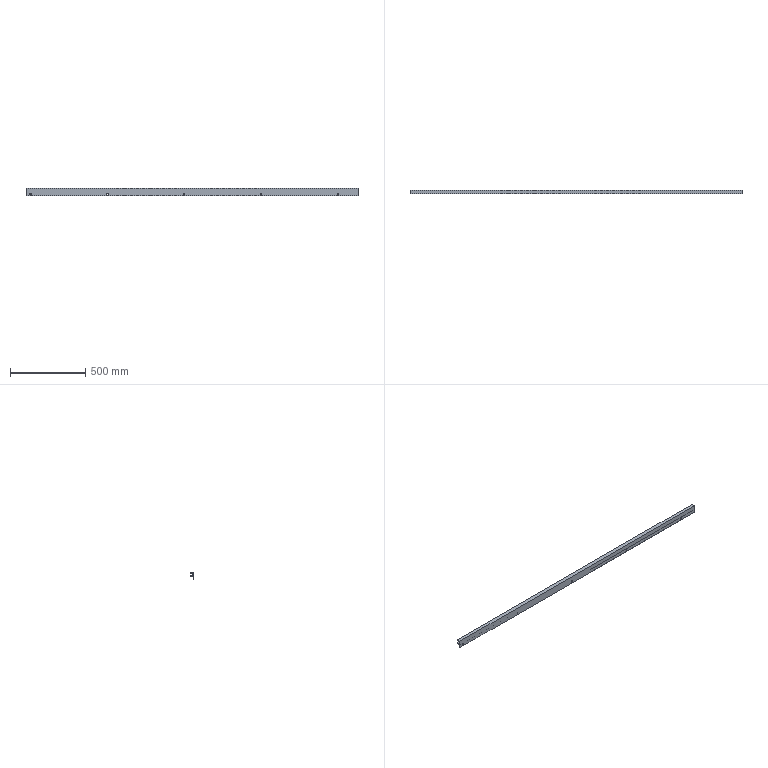Part | SolidWorks | features ICE 3, Extrusion 1, LPattern 1 | 1 solid | 45 faces | box 2200 x 24 x 52 mm | volume 1222839 mm3 | plane 30 | cylinder 15 | commonest cylinder face diameters 7 x15
STEP:
#1=CARTESIAN_POINT('',(540.,-9.,-33.5));
#2=VERTEX_POINT('',#1);
#3=CARTESIAN_POINT('',(543.5,-9.,-30.));
#4=VERTEX_POINT('',#3);
#5=CARTESIAN_POINT('',(540.,-9.,-30.));
#6=DIRECTION('',(0.,-1.,0.));
#7=DIRECTION('',(0.,0.,-1.));
#8=AXIS2_PLACEMENT_3D('',#5,#6,#7);
#9=CIRCLE('',#8,3.5);
#10=EDGE_CURVE('',#2,#4,#9,.T.);
#11=ORIENTED_EDGE('',*,*,#10,.F.);
#12=CARTESIAN_POINT('',(540.,-12.,-33.5));
#13=VERTEX_POINT('',#12);
#14=CARTESIAN_POINT('',(540.,10.,-33.5));
#15=DIRECTION('',(0.,-1.,0.));
#16=VECTOR('',#15,1000.);
#17=LINE('',#14,#16);
#18=EDGE_CURVE('',#2,#13,#17,.T.);
#19=ORIENTED_EDGE('',*,*,#18,.T.);
#20=CARTESIAN_POINT('',(543.5,-12.,-30.));
#21=VERTEX_POINT('',#20);
#22=CARTESIAN_POINT('',(540.,-12.,-30.));
#23=DIRECTION('',(0.,-1.,0.));
#24=DIRECTION('',(0.,0.,-1.));
#25=AXIS2_PLACEMENT_3D('',#22,#23,#24);
#26=CIRCLE('',#25,3.5);
#27=EDGE_CURVE('',#13,#21,#26,.T.);
#28=ORIENTED_EDGE('',*,*,#27,.T.);
#29=CARTESIAN_POINT('',(543.5,10.,-30.));
#30=DIRECTION('',(0.,-1.,0.));
#31=VECTOR('',#30,1000.);
#32=LINE('',#29,#31);
#33=EDGE_CURVE('',#4,#21,#32,.T.);
#34=ORIENTED_EDGE('',*,*,#33,.F.);
#35=EDGE_LOOP('',(#11,#19,#28,#34));
#36=FACE_OUTER_BOUND('',#35,.T.);
#37=CARTESIAN_POINT('',(540.,10.,-30.));
#38=DIRECTION('',(0.,-1.,0.));
#39=DIRECTION('',(0.,0.,-1.));
#40=AXIS2_PLACEMENT_3D('',#37,#38,#39);
#41=CYLINDRICAL_SURFACE('',#40,3.5);
#42=ADVANCED_FACE('',(#36),#41,.F.);
#43=CARTESIAN_POINT('',(1050.,-9.,-33.5));
#44=VERTEX_POINT('',#43);
#45=CARTESIAN_POINT('',(1053.5,-9.,-30.));
#46=VERTEX_POINT('',#45);
#47=CARTESIAN_POINT('',(1050.,-9.,-30.));
#48=DIRECTION('',(0.,-1.,0.));
#49=DIRECTION('',(0.,0.,-1.));
#50=AXIS2_PLACEMENT_3D('',#47,#48,#49);
#51=CIRCLE('',#50,3.5);
#52=EDGE_CURVE('',#44,#46,#51,.T.);
#53=ORIENTED_EDGE('',*,*,#52,.F.);
#54=CARTESIAN_POINT('',(1050.,-12.,-33.5));
#55=VERTEX_POINT('',#54);
#56=CARTESIAN_POINT('',(1050.,10.,-33.5));
#57=DIRECTION('',(0.,-1.,0.));
#58=VECTOR('',#57,1000.);
#59=LINE('',#56,#58);
#60=EDGE_CURVE('',#44,#55,#59,.T.);
#61=ORIENTED_EDGE('',*,*,#60,.T.);
#62=CARTESIAN_POINT('',(1053.5,-12.,-30.));
#63=VERTEX_POINT('',#62);
#64=CARTESIAN_POINT('',(1050.,-12.,-30.));
#65=DIRECTION('',(0.,-1.,0.));
#66=DIRECTION('',(0.,0.,-1.));
#67=AXIS2_PLACEMENT_3D('',#64,#65,#66);
#68=CIRCLE('',#67,3.5);
#69=EDGE_CURVE('',#55,#63,#68,.T.);
#70=ORIENTED_EDGE('',*,*,#69,.T.);
#71=CARTESIAN_POINT('',(1053.5,10.,-30.));
#72=DIRECTION('',(0.,-1.,0.));
#73=VECTOR('',#72,1000.);
#74=LINE('',#71,#73);
#75=EDGE_CURVE('',#46,#63,#74,.T.);
#76=ORIENTED_EDGE('',*,*,#75,.F.);
#77=EDGE_LOOP('',(#53,#61,#70,#76));
#78=FACE_OUTER_BOUND('',#77,.T.);
#79=CARTESIAN_POINT('',(1050.,10.,-30.));
#80=DIRECTION('',(0.,-1.,0.));
#81=DIRECTION('',(0.,0.,-1.));
#82=AXIS2_PLACEMENT_3D('',#79,#80,#81);
#83=CYLINDRICAL_SURFACE('',#82,3.5);
#84=ADVANCED_FACE('',(#78),#83,.F.);
#85=CARTESIAN_POINT('',(1560.,-9.,-33.5));
#86=VERTEX_POINT('',#85);
#87=CARTESIAN_POINT('',(1563.5,-9.,-30.));
#88=VERTEX_POINT('',#87);
#89=CARTESIAN_POINT('',(1560.,-9.,-30.));
#90=DIRECTION('',(0.,-1.,0.));
#91=DIRECTION('',(0.,0.,-1.));
#92=AXIS2_PLACEMENT_3D('',#89,#90,#91);
#93=CIRCLE('',#92,3.5);
#94=EDGE_CURVE('',#86,#88,#93,.T.);
#95=ORIENTED_EDGE('',*,*,#94,.F.);
#96=CARTESIAN_POINT('',(1560.,-12.,-33.5));
#97=VERTEX_POINT('',#96);
#98=CARTESIAN_POINT('',(1560.,10.,-33.5));
#99=DIRECTION('',(0.,-1.,0.));
#100=VECTOR('',#99,1000.);
#101=LINE('',#98,#100);
#102=EDGE_CURVE('',#86,#97,#101,.T.);
#103=ORIENTED_EDGE('',*,*,#102,.T.);
#104=CARTESIAN_POINT('',(1563.5,-12.,-30.));
#105=VERTEX_POINT('',#104);
#106=CARTESIAN_POINT('',(1560.,-12.,-30.));
#107=DIRECTION('',(0.,-1.,0.));
#108=DIRECTION('',(0.,0.,-1.));
#109=AXIS2_PLACEMENT_3D('',#106,#107,#108);
#110=CIRCLE('',#109,3.5);
#111=EDGE_CURVE('',#97,#105,#110,.T.);
#112=ORIENTED_EDGE('',*,*,#111,.T.);
#113=CARTESIAN_POINT('',(1563.5,10.,-30.));
#114=DIRECTION('',(0.,-1.,0.));
#115=VECTOR('',#114,1000.);
#116=LINE('',#113,#115);
#117=EDGE_CURVE('',#88,#105,#116,.T.);
#118=ORIENTED_EDGE('',*,*,#117,.F.);
#119=EDGE_LOOP('',(#95,#103,#112,#118));
#120=FACE_OUTER_BOUND('',#119,.T.);
#121=CARTESIAN_POINT('',(1560.,10.,-30.));
#122=DIRECTION('',(0.,-1.,0.));
#123=DIRECTION('',(0.,0.,-1.));
#124=AXIS2_PLACEMENT_3D('',#121,#122,#123);
#125=CYLINDRICAL_SURFACE('',#124,3.5);
#126=ADVANCED_FACE('',(#120),#125,.F.);
#127=CARTESIAN_POINT('',(2070.,-9.,-33.5));
#128=VERTEX_POINT('',#127);
#129=CARTESIAN_POINT('',(2073.5,-9.,-30.));
#130=VERTEX_POINT('',#129);
#131=CARTESIAN_POINT('',(2070.,-9.,-30.));
#132=DIRECTION('',(0.,-1.,0.));
#133=DIRECTION('',(0.,0.,-1.));
#134=AXIS2_PLACEMENT_3D('',#131,#132,#133);
#135=CIRCLE('',#134,3.5);
#136=EDGE_CURVE('',#128,#130,#135,.T.);
#137=ORIENTED_EDGE('',*,*,#136,.F.);
#138=CARTESIAN_POINT('',(2070.,-12.,-33.5));
#139=VERTEX_POINT('',#138);
#140=CARTESIAN_POINT('',(2070.,10.,-33.5));
#141=DIRECTION('',(0.,-1.,0.));
#142=VECTOR('',#141,1000.);
#143=LINE('',#140,#142);
#144=EDGE_CURVE('',#128,#139,#143,.T.);
#145=ORIENTED_EDGE('',*,*,#144,.T.);
#146=CARTESIAN_POINT('',(2073.5,-12.,-30.));
#147=VERTEX_POINT('',#146);
#148=CARTESIAN_POINT('',(2070.,-12.,-30.));
#149=DIRECTION('',(0.,-1.,0.));
#150=DIRECTION('',(0.,0.,-1.));
#151=AXIS2_PLACEMENT_3D('',#148,#149,#150);
#152=CIRCLE('',#151,3.5);
#153=EDGE_CURVE('',#139,#147,#152,.T.);
#154=ORIENTED_EDGE('',*,*,#153,.T.);
#155=CARTESIAN_POINT('',(2073.5,10.,-30.));
#156=DIRECTION('',(0.,-1.,0.));
#157=VECTOR('',#156,1000.);
#158=LINE('',#155,#157);
#159=EDGE_CURVE('',#130,#147,#158,.T.);
#160=ORIENTED_EDGE('',*,*,#159,.F.);
#161=EDGE_LOOP('',(#137,#145,#154,#160));
#162=FACE_OUTER_BOUND('',#161,.T.);
#163=CARTESIAN_POINT('',(2070.,10.,-30.));
#164=DIRECTION('',(0.,-1.,0.));
#165=DIRECTION('',(0.,0.,-1.));
#166=AXIS2_PLACEMENT_3D('',#163,#164,#165);
#167=CYLINDRICAL_SURFACE('',#166,3.5);
#168=ADVANCED_FACE('',(#162),#167,.F.);
#169=CARTESIAN_POINT('',(30.,-9.,-33.5));
#170=VERTEX_POINT('',#169);
#171=CARTESIAN_POINT('',(33.5,-9.,-30.));
#172=VERTEX_POINT('',#171);
#173=CARTESIAN_POINT('',(30.,-9.,-30.));
#174=DIRECTION('',(0.,-1.,0.));
#175=DIRECTION('',(0.,0.,-1.));
#176=AXIS2_PLACEMENT_3D('',#173,#174,#175);
#177=CIRCLE('',#176,3.5);
#178=EDGE_CURVE('',#170,#172,#177,.T.);
#179=ORIENTED_EDGE('',*,*,#178,.F.);
#180=CARTESIAN_POINT('',(30.,-12.,-33.5));
#181=VERTEX_POINT('',#180);
#182=CARTESIAN_POINT('',(30.,10.,-33.5));
#183=DIRECTION('',(0.,-1.,0.));
#184=VECTOR('',#183,1000.);
#185=LINE('',#182,#184);
#186=EDGE_CURVE('',#170,#181,#185,.T.);
#187=ORIENTED_EDGE('',*,*,#186,.T.);
#188=CARTESIAN_POINT('',(33.5,-12.,-30.));
#189=VERTEX_POINT('',#188);
#190=CARTESIAN_POINT('',(30.,-12.,-30.));
#191=DIRECTION('',(0.,-1.,0.));
#192=DIRECTION('',(0.,0.,-1.));
#193=AXIS2_PLACEMENT_3D('',#190,#191,#192);
#194=CIRCLE('',#193,3.5);
#195=EDGE_CURVE('',#181,#189,#194,.T.);
#196=ORIENTED_EDGE('',*,*,#195,.T.);
#197=CARTESIAN_POINT('',(33.5,10.,-30.));
#198=DIRECTION('',(0.,-1.,0.));
#199=VECTOR('',#198,1000.);
#200=LINE('',#197,#199);
#201=EDGE_CURVE('',#172,#189,#200,.T.);
#202=ORIENTED_EDGE('',*,*,#201,.F.);
#203=EDGE_LOOP('',(#179,#187,#196,#202));
#204=FACE_OUTER_BOUND('',#203,.T.);
#205=CARTESIAN_POINT('',(30.,10.,-30.));
#206=DIRECTION('',(0.,-1.,0.));
#207=DIRECTION('',(0.,0.,-1.));
#208=AXIS2_PLACEMENT_3D('',#205,#206,#207);
#209=CYLINDRICAL_SURFACE('',#208,3.5);
#210=ADVANCED_FACE('',(#204),#209,.F.);
#211=CARTESIAN_POINT('',(0.,-9.,-15.));
#212=VERTEX_POINT('',#211);
#213=CARTESIAN_POINT('',(2200.,-9.,-15.));
#214=VERTEX_POINT('',#213);
#215=CARTESIAN_POINT('',(2200.,-9.,-15.));
#216=DIRECTION('',(1.,0.,0.));
#217=VECTOR('',#216,1000.);
#218=LINE('',#215,#217);
#219=EDGE_CURVE('',#212,#214,#218,.T.);
#220=ORIENTED_EDGE('',*,*,#219,.F.);
#221=CARTESIAN_POINT('',(0.,12.,-15.));
#222=VERTEX_POINT('',#221);
#223=CARTESIAN_POINT('',(0.,12.,-15.));
#224=DIRECTION('',(0.,1.,0.));
#225=VECTOR('',#224,1000.);
#226=LINE('',#223,#225);
#227=EDGE_CURVE('',#212,#222,#226,.T.);
#228=ORIENTED_EDGE('',*,*,#227,.T.);
#229=CARTESIAN_POINT('',(2200.,12.,-15.));
#230=VERTEX_POINT('',#229);
#231=CARTESIAN_POINT('',(2200.,12.,-15.));
#232=DIRECTION('',(-1.,0.,0.));
#233=VECTOR('',#232,1000.);
#234=LINE('',#231,#233);
#235=EDGE_CURVE('',#230,#222,#234,.T.);
#236=ORIENTED_EDGE('',*,*,#235,.F.);
#237=CARTESIAN_POINT('',(2200.,12.,-15.));
#238=DIRECTION('',(0.,1.,0.));
#239=VECTOR('',#238,1000.);
#240=LINE('',#237,#239);
#241=EDGE_CURVE('',#214,#230,#240,.T.);
#242=ORIENTED_EDGE('',*,*,#241,.F.);
#243=EDGE_LOOP('',(#220,#228,#236,#242));
#244=FACE_OUTER_BOUND('',#243,.T.);
#245=CARTESIAN_POINT('',(2200.,12.,-15.));
#246=DIRECTION('',(0.,0.,1.));
#247=DIRECTION('',(0.,-1.,0.));
#248=AXIS2_PLACEMENT_3D('',#245,#246,#247);
#249=PLANE('',#248);
#250=ADVANCED_FACE('',(#244),#249,.F.);
#251=CARTESIAN_POINT('',(0.,12.,-6.2));
#252=VERTEX_POINT('',#251);
#253=CARTESIAN_POINT('',(2200.,12.,-6.2));
#254=VERTEX_POINT('',#253);
#255=CARTESIAN_POINT('',(0.,12.,-6.2));
#256=DIRECTION('',(1.,0.,0.));
#257=VECTOR('',#256,1000.);
#258=LINE('',#255,#257);
#259=EDGE_CURVE('',#252,#254,#258,.T.);
#260=ORIENTED_EDGE('',*,*,#259,.T.);
#261=CARTESIAN_POINT('',(2200.,12.,15.));
#262=DIRECTION('',(0.,0.,1.));
#263=VECTOR('',#262,1000.);
#264=LINE('',#261,#263);
#265=EDGE_CURVE('',#230,#254,#264,.T.);
#266=ORIENTED_EDGE('',*,*,#265,.F.);
#267=ORIENTED_EDGE('',*,*,#235,.T.);
#268=CARTESIAN_POINT('',(0.,12.,15.));
#269=DIRECTION('',(0.,0.,1.));
#270=VECTOR('',#269,1000.);
#271=LINE('',#268,#270);
#272=EDGE_CURVE('',#222,#252,#271,.T.);
#273=ORIENTED_EDGE('',*,*,#272,.T.);
#274=EDGE_LOOP('',(#260,#266,#267,#273));
#275=FACE_OUTER_BOUND('',#274,.T.);
#276=CARTESIAN_POINT('',(2200.,12.,15.));
#277=DIRECTION('',(0.,-1.,0.));
#278=DIRECTION('',(0.,0.,-1.));
#279=AXIS2_PLACEMENT_3D('',#276,#277,#278);
#280=PLANE('',#279);
#281=ADVANCED_FACE('',(#275),#280,.F.);
#282=ORIENTED_EDGE('',*,*,#265,.T.);
#283=CARTESIAN_POINT('',(2200.,0.7,-6.2));
#284=VERTEX_POINT('',#283);
#285=CARTESIAN_POINT('',(2200.,12.,-6.2));
#286=DIRECTION('',(0.,-1.,0.));
#287=VECTOR('',#286,1000.);
#288=LINE('',#285,#287);
#289=EDGE_CURVE('',#254,#284,#288,.T.);
#290=ORIENTED_EDGE('',*,*,#289,.T.);
#291=CARTESIAN_POINT('',(2200.,0.7,-8.5));
#292=VERTEX_POINT('',#291);
#293=CARTESIAN_POINT('',(2200.,0.7,-6.2));
#294=DIRECTION('',(0.,0.,-1.));
#295=VECTOR('',#294,1000.);
#296=LINE('',#293,#295);
#297=EDGE_CURVE('',#284,#292,#296,.T.);
#298=ORIENTED_EDGE('',*,*,#297,.T.);
#299=CARTESIAN_POINT('',(2200.,-3.9,-8.5));
#300=VERTEX_POINT('',#299);
#301=CARTESIAN_POINT('',(2200.,0.7,-8.5));
#302=DIRECTION('',(0.,-1.,0.));
#303=VECTOR('',#302,1000.);
#304=LINE('',#301,#303);
#305=EDGE_CURVE('',#292,#300,#304,.T.);
#306=ORIENTED_EDGE('',*,*,#305,.T.);
#307=CARTESIAN_POINT('',(2200.,-3.9,-3.5));
#308=VERTEX_POINT('',#307);
#309=CARTESIAN_POINT('',(2200.,-3.9,-8.5));
#310=DIRECTION('',(0.,0.,1.));
#311=VECTOR('',#310,1000.);
#312=LINE('',#309,#311);
#313=EDGE_CURVE('',#300,#308,#312,.T.);
#314=ORIENTED_EDGE('',*,*,#313,.T.);
#315=CARTESIAN_POINT('',(2200.,-5.5,-3.5));
#316=VERTEX_POINT('',#315);
#317=CARTESIAN_POINT('',(2200.,-3.9,-3.5));
#318=DIRECTION('',(0.,-1.,0.));
#319=VECTOR('',#318,1000.);
#320=LINE('',#317,#319);
#321=EDGE_CURVE('',#308,#316,#320,.T.);
#322=ORIENTED_EDGE('',*,*,#321,.T.);
#323=CARTESIAN_POINT('',(2200.,-5.5,3.5));
#324=VERTEX_POINT('',#323);
#325=CARTESIAN_POINT('',(2200.,-5.5,3.5));
#326=DIRECTION('',(0.,0.,-1.));
#327=VECTOR('',#326,1000.);
#328=LINE('',#325,#327);
#329=EDGE_CURVE('',#324,#316,#328,.T.);
#330=ORIENTED_EDGE('',*,*,#329,.F.);
#331=CARTESIAN_POINT('',(2200.,-3.9,3.5));
#332=VERTEX_POINT('',#331);
#333=CARTESIAN_POINT('',(2200.,-3.9,3.5));
#334=DIRECTION('',(0.,-1.,0.));
#335=VECTOR('',#334,1000.);
#336=LINE('',#333,#335);
#337=EDGE_CURVE('',#332,#324,#336,.T.);
#338=ORIENTED_EDGE('',*,*,#337,.F.);
#339=CARTESIAN_POINT('',(2200.,-3.9,8.5));
#340=VERTEX_POINT('',#339);
#341=CARTESIAN_POINT('',(2200.,-3.9,8.5));
#342=DIRECTION('',(0.,0.,-1.));
#343=VECTOR('',#342,1000.);
#344=LINE('',#341,#343);
#345=EDGE_CURVE('',#340,#332,#344,.T.);
#346=ORIENTED_EDGE('',*,*,#345,.F.);
#347=CARTESIAN_POINT('',(2200.,0.7,8.5));
#348=VERTEX_POINT('',#347);
#349=CARTESIAN_POINT('',(2200.,0.7,8.5));
#350=DIRECTION('',(0.,-1.,0.));
#351=VECTOR('',#350,1000.);
#352=LINE('',#349,#351);
#353=EDGE_CURVE('',#348,#340,#352,.T.);
#354=ORIENTED_EDGE('',*,*,#353,.F.);
#355=CARTESIAN_POINT('',(2200.,0.7,6.2));
#356=VERTEX_POINT('',#355);
#357=CARTESIAN_POINT('',(2200.,0.7,6.2));
#358=DIRECTION('',(0.,0.,1.));
#359=VECTOR('',#358,1000.);
#360=LINE('',#357,#359);
#361=EDGE_CURVE('',#356,#348,#360,.T.);
#362=ORIENTED_EDGE('',*,*,#361,.F.);
#363=CARTESIAN_POINT('',(2200.,12.,6.2));
#364=VERTEX_POINT('',#363);
#365=CARTESIAN_POINT('',(2200.,12.,6.2));
#366=DIRECTION('',(0.,-1.,0.));
#367=VECTOR('',#366,1000.);
#368=LINE('',#365,#367);
#369=EDGE_CURVE('',#364,#356,#368,.T.);
#370=ORIENTED_EDGE('',*,*,#369,.F.);
#371=CARTESIAN_POINT('',(2200.,12.,15.));
#372=VERTEX_POINT('',#371);
#373=CARTESIAN_POINT('',(2200.,12.,15.));
#374=DIRECTION('',(0.,0.,1.));
#375=VECTOR('',#374,1000.);
#376=LINE('',#373,#375);
#377=EDGE_CURVE('',#364,#372,#376,.T.);
#378=ORIENTED_EDGE('',*,*,#377,.T.);
#379=CARTESIAN_POINT('',(2200.,-12.,15.));
#380=VERTEX_POINT('',#379);
#381=CARTESIAN_POINT('',(2200.,12.,15.));
#382=DIRECTION('',(0.,-1.,0.));
#383=VECTOR('',#382,1000.);
#384=LINE('',#381,#383);
#385=EDGE_CURVE('',#372,#380,#384,.T.);
#386=ORIENTED_EDGE('',*,*,#385,.T.);
#387=CARTESIAN_POINT('',(2200.,-12.,-37.));
#388=VERTEX_POINT('',#387);
#389=CARTESIAN_POINT('',(2200.,-12.,15.));
#390=DIRECTION('',(0.,0.,-1.));
#391=VECTOR('',#390,1000.);
#392=LINE('',#389,#391);
#393=EDGE_CURVE('',#380,#388,#392,.T.);
#394=ORIENTED_EDGE('',*,*,#393,.T.);
#395=CARTESIAN_POINT('',(2200.,-9.,-37.));
#396=VERTEX_POINT('',#395);
#397=CARTESIAN_POINT('',(2200.,-12.,-37.));
#398=DIRECTION('',(0.,-1.,0.));
#399=VECTOR('',#398,1000.);
#400=LINE('',#397,#399);
#401=EDGE_CURVE('',#396,#388,#400,.T.);
#402=ORIENTED_EDGE('',*,*,#401,.F.);
#403=CARTESIAN_POINT('',(2200.,-9.,-37.));
#404=DIRECTION('',(0.,0.,1.));
#405=VECTOR('',#404,1000.);
#406=LINE('',#403,#405);
#407=EDGE_CURVE('',#396,#214,#406,.T.);
#408=ORIENTED_EDGE('',*,*,#407,.T.);
#409=ORIENTED_EDGE('',*,*,#241,.T.);
#410=EDGE_LOOP('',(#282,#290,#298,#306,#314,#322,#330,#338,#346,#354,#362,#370,#378,#386,#394,#402,#408,#409));
#411=FACE_OUTER_BOUND('',#410,.T.);
#412=CARTESIAN_POINT('',(2200.,0.,0.));
#413=DIRECTION('',(1.,0.,0.));
#414=DIRECTION('',(0.,0.,-1.));
#415=AXIS2_PLACEMENT_3D('',#412,#413,#414);
#416=PLANE('',#415);
#417=ADVANCED_FACE('',(#411),#416,.T.);
#418=CARTESIAN_POINT('',(0.,0.7,-6.2));
#419=VERTEX_POINT('',#418);
#420=CARTESIAN_POINT('',(0.,12.,-6.2));
#421=DIRECTION('',(0.,-1.,0.));
#422=VECTOR('',#421,1000.);
#423=LINE('',#420,#422);
#424=EDGE_CURVE('',#252,#419,#423,.T.);
#425=ORIENTED_EDGE('',*,*,#424,.F.);
#426=ORIENTED_EDGE('',*,*,#272,.F.);
#427=ORIENTED_EDGE('',*,*,#227,.F.);
#428=CARTESIAN_POINT('',(0.,-9.,-37.));
#429=VERTEX_POINT('',#428);
#430=CARTESIAN_POINT('',(0.,-9.,-37.));
#431=DIRECTION('',(0.,0.,1.));
#432=VECTOR('',#431,1000.);
#433=LINE('',#430,#432);
#434=EDGE_CURVE('',#429,#212,#433,.T.);
#435=ORIENTED_EDGE('',*,*,#434,.F.);
#436=CARTESIAN_POINT('',(0.,-12.,-37.));
#437=VERTEX_POINT('',#436);
#438=CARTESIAN_POINT('',(0.,-12.,-37.));
#439=DIRECTION('',(0.,1.,0.));
#440=VECTOR('',#439,1000.);
#441=LINE('',#438,#440);
#442=EDGE_CURVE('',#437,#429,#441,.T.);
#443=ORIENTED_EDGE('',*,*,#442,.F.);
#444=CARTESIAN_POINT('',(0.,-12.,15.));
#445=VERTEX_POINT('',#444);
#446=CARTESIAN_POINT('',(0.,-12.,15.));
#447=DIRECTION('',(0.,0.,-1.));
#448=VECTOR('',#447,1000.);
#449=LINE('',#446,#448);
#450=EDGE_CURVE('',#445,#437,#449,.T.);
#451=ORIENTED_EDGE('',*,*,#450,.F.);
#452=CARTESIAN_POINT('',(0.,12.,15.));
#453=VERTEX_POINT('',#452);
#454=CARTESIAN_POINT('',(0.,12.,15.));
#455=DIRECTION('',(0.,-1.,0.));
#456=VECTOR('',#455,1000.);
#457=LINE('',#454,#456);
#458=EDGE_CURVE('',#453,#445,#457,.T.);
#459=ORIENTED_EDGE('',*,*,#458,.F.);
#460=CARTESIAN_POINT('',(0.,12.,6.2));
#461=VERTEX_POINT('',#460);
#462=CARTESIAN_POINT('',(0.,12.,15.));
#463=DIRECTION('',(0.,0.,1.));
#464=VECTOR('',#463,1000.);
#465=LINE('',#462,#464);
#466=EDGE_CURVE('',#461,#453,#465,.T.);
#467=ORIENTED_EDGE('',*,*,#466,.F.);
#468=CARTESIAN_POINT('',(0.,0.7,6.2));
#469=VERTEX_POINT('',#468);
#470=CARTESIAN_POINT('',(0.,12.,6.2));
#471=DIRECTION('',(0.,-1.,0.));
#472=VECTOR('',#471,1000.);
#473=LINE('',#470,#472);
#474=EDGE_CURVE('',#461,#469,#473,.T.);
#475=ORIENTED_EDGE('',*,*,#474,.T.);
#476=CARTESIAN_POINT('',(0.,0.7,8.5));
#477=VERTEX_POINT('',#476);
#478=CARTESIAN_POINT('',(0.,0.7,6.2));
#479=DIRECTION('',(0.,0.,1.));
#480=VECTOR('',#479,1000.);
#481=LINE('',#478,#480);
#482=EDGE_CURVE('',#469,#477,#481,.T.);
#483=ORIENTED_EDGE('',*,*,#482,.T.);
#484=CARTESIAN_POINT('',(0.,-3.9,8.5));
#485=VERTEX_POINT('',#484);
#486=CARTESIAN_POINT('',(0.,0.7,8.5));
#487=DIRECTION('',(0.,-1.,0.));
#488=VECTOR('',#487,1000.);
#489=LINE('',#486,#488);
#490=EDGE_CURVE('',#477,#485,#489,.T.);
#491=ORIENTED_EDGE('',*,*,#490,.T.);
#492=CARTESIAN_POINT('',(0.,-3.9,3.5));
#493=VERTEX_POINT('',#492);
#494=CARTESIAN_POINT('',(0.,-3.9,8.5));
#495=DIRECTION('',(0.,0.,-1.));
#496=VECTOR('',#495,1000.);
#497=LINE('',#494,#496);
#498=EDGE_CURVE('',#485,#493,#497,.T.);
#499=ORIENTED_EDGE('',*,*,#498,.T.);
#500=CARTESIAN_POINT('',(0.,-5.5,3.5));
#501=VERTEX_POINT('',#500);
#502=CARTESIAN_POINT('',(0.,-3.9,3.5));
#503=DIRECTION('',(0.,-1.,0.));
#504=VECTOR('',#503,1000.);
#505=LINE('',#502,#504);
#506=EDGE_CURVE('',#493,#501,#505,.T.);
#507=ORIENTED_EDGE('',*,*,#506,.T.);
#508=CARTESIAN_POINT('',(0.,-5.5,-3.5));
#509=VERTEX_POINT('',#508);
#510=CARTESIAN_POINT('',(0.,-5.5,3.5));
#511=DIRECTION('',(0.,0.,-1.));
#512=VECTOR('',#511,1000.);
#513=LINE('',#510,#512);
#514=EDGE_CURVE('',#501,#509,#513,.T.);
#515=ORIENTED_EDGE('',*,*,#514,.T.);
#516=CARTESIAN_POINT('',(0.,-3.9,-3.5));
#517=VERTEX_POINT('',#516);
#518=CARTESIAN_POINT('',(0.,-3.9,-3.5));
#519=DIRECTION('',(0.,-1.,0.));
#520=VECTOR('',#519,1000.);
#521=LINE('',#518,#520);
#522=EDGE_CURVE('',#517,#509,#521,.T.);
#523=ORIENTED_EDGE('',*,*,#522,.F.);
#524=CARTESIAN_POINT('',(0.,-3.9,-8.5));
#525=VERTEX_POINT('',#524);
#526=CARTESIAN_POINT('',(0.,-3.9,-8.5));
#527=DIRECTION('',(0.,0.,1.));
#528=VECTOR('',#527,1000.);
#529=LINE('',#526,#528);
#530=EDGE_CURVE('',#525,#517,#529,.T.);
#531=ORIENTED_EDGE('',*,*,#530,.F.);
#532=CARTESIAN_POINT('',(0.,0.7,-8.5));
#533=VERTEX_POINT('',#532);
#534=CARTESIAN_POINT('',(0.,0.7,-8.5));
#535=DIRECTION('',(0.,-1.,0.));
#536=VECTOR('',#535,1000.);
#537=LINE('',#534,#536);
#538=EDGE_CURVE('',#533,#525,#537,.T.);
#539=ORIENTED_EDGE('',*,*,#538,.F.);
#540=CARTESIAN_POINT('',(0.,0.7,-6.2));
#541=DIRECTION('',(0.,0.,-1.));
#542=VECTOR('',#541,1000.);
#543=LINE('',#540,#542);
#544=EDGE_CURVE('',#419,#533,#543,.T.);
#545=ORIENTED_EDGE('',*,*,#544,.F.);
#546=EDGE_LOOP('',(#425,#426,#427,#435,#443,#451,#459,#467,#475,#483,#491,#499,#507,#515,#523,#531,#539,#545));
#547=FACE_OUTER_BOUND('',#546,.T.);
#548=CARTESIAN_POINT('',(0.,0.,0.));
#549=DIRECTION('',(1.,0.,0.));
#550=DIRECTION('',(0.,0.,-1.));
#551=AXIS2_PLACEMENT_3D('',#548,#549,#550);
#552=PLANE('',#551);
#553=ADVANCED_FACE('',(#547),#552,.F.);
#554=ORIENTED_EDGE('',*,*,#377,.F.);
#555=CARTESIAN_POINT('',(0.,12.,6.2));
#556=DIRECTION('',(1.,0.,0.));
#557=VECTOR('',#556,1000.);
#558=LINE('',#555,#557);
#559=EDGE_CURVE('',#461,#364,#558,.T.);
#560=ORIENTED_EDGE('',*,*,#559,.F.);
#561=ORIENTED_EDGE('',*,*,#466,.T.);
#562=CARTESIAN_POINT('',(2200.,12.,15.));
#563=DIRECTION('',(-1.,0.,0.));
#564=VECTOR('',#563,1000.);
#565=LINE('',#562,#564);
#566=EDGE_CURVE('',#372,#453,#565,.T.);
#567=ORIENTED_EDGE('',*,*,#566,.F.);
#568=EDGE_LOOP('',(#554,#560,#561,#567));
#569=FACE_OUTER_BOUND('',#568,.T.);
#570=CARTESIAN_POINT('',(2200.,12.,15.));
#571=DIRECTION('',(0.,-1.,0.));
#572=DIRECTION('',(0.,0.,-1.));
#573=AXIS2_PLACEMENT_3D('',#570,#571,#572);
#574=PLANE('',#573);
#575=ADVANCED_FACE('',(#569),#574,.F.);
#576=ORIENTED_EDGE('',*,*,#458,.T.);
#577=CARTESIAN_POINT('',(2200.,-12.,15.));
#578=DIRECTION('',(-1.,0.,0.));
#579=VECTOR('',#578,1000.);
#580=LINE('',#577,#579);
#581=EDGE_CURVE('',#380,#445,#580,.T.);
#582=ORIENTED_EDGE('',*,*,#581,.F.);
#583=ORIENTED_EDGE('',*,*,#385,.F.);
#584=ORIENTED_EDGE('',*,*,#566,.T.);
#585=EDGE_LOOP('',(#576,#582,#583,#584));
#586=FACE_OUTER_BOUND('',#585,.T.);
#587=CARTESIAN_POINT('',(2200.,12.,15.));
#588=DIRECTION('',(0.,0.,-1.));
#589=DIRECTION('',(0.,1.,0.));
#590=AXIS2_PLACEMENT_3D('',#587,#588,#589);
#591=PLANE('',#590);
#592=ADVANCED_FACE('',(#586),#591,.F.);
#593=CARTESIAN_POINT('',(536.5,-12.,-22.));
#594=VERTEX_POINT('',#593);
#595=CARTESIAN_POINT('',(536.5,-12.,-30.));
#596=VERTEX_POINT('',#595);
#597=CARTESIAN_POINT('',(536.5,-12.,-22.));
#598=DIRECTION('',(0.,0.,-1.));
#599=VECTOR('',#598,1000.);
#600=LINE('',#597,#599);
#601=EDGE_CURVE('',#594,#596,#600,.T.);
#602=ORIENTED_EDGE('',*,*,#601,.F.);
#603=CARTESIAN_POINT('',(543.5,-12.,-22.));
#604=VERTEX_POINT('',#603);
#605=CARTESIAN_POINT('',(540.,-12.,-22.));
#606=DIRECTION('',(0.,-1.,0.));
#607=DIRECTION('',(0.,0.,-1.));
#608=AXIS2_PLACEMENT_3D('',#605,#606,#607);
#609=CIRCLE('',#608,3.5);
#610=EDGE_CURVE('',#604,#594,#609,.T.);
#611=ORIENTED_EDGE('',*,*,#610,.F.);
#612=CARTESIAN_POINT('',(543.5,-12.,-22.));
#613=DIRECTION('',(0.,0.,1.));
#614=VECTOR('',#613,1000.);
#615=LINE('',#612,#614);
#616=EDGE_CURVE('',#21,#604,#615,.T.);
#617=ORIENTED_EDGE('',*,*,#616,.F.);
#618=ORIENTED_EDGE('',*,*,#27,.F.);
#619=CARTESIAN_POINT('',(540.,-12.,-30.));
#620=DIRECTION('',(0.,-1.,0.));
#621=DIRECTION('',(0.,0.,-1.));
#622=AXIS2_PLACEMENT_3D('',#619,#620,#621);
#623=CIRCLE('',#622,3.5);
#624=EDGE_CURVE('',#596,#13,#623,.T.);
#625=ORIENTED_EDGE('',*,*,#624,.F.);
#626=EDGE_LOOP('',(#602,#611,#617,#618,#625));
#627=FACE_BOUND('',#626,.T.);
#628=CARTESIAN_POINT('',(1046.5,-12.,-22.));
#629=VERTEX_POINT('',#628);
#630=CARTESIAN_POINT('',(1046.5,-12.,-30.));
#631=VERTEX_POINT('',#630);
#632=CARTESIAN_POINT('',(1046.5,-12.,-22.));
#633=DIRECTION('',(0.,0.,-1.));
#634=VECTOR('',#633,1000.);
#635=LINE('',#632,#634);
#636=EDGE_CURVE('',#629,#631,#635,.T.);
#637=ORIENTED_EDGE('',*,*,#636,.F.);
#638=CARTESIAN_POINT('',(1053.5,-12.,-22.));
#639=VERTEX_POINT('',#638);
#640=CARTESIAN_POINT('',(1050.,-12.,-22.));
#641=DIRECTION('',(0.,-1.,0.));
#642=DIRECTION('',(0.,0.,-1.));
#643=AXIS2_PLACEMENT_3D('',#640,#641,#642);
#644=CIRCLE('',#643,3.5);
#645=EDGE_CURVE('',#639,#629,#644,.T.);
#646=ORIENTED_EDGE('',*,*,#645,.F.);
#647=CARTESIAN_POINT('',(1053.5,-12.,-22.));
#648=DIRECTION('',(0.,0.,1.));
#649=VECTOR('',#648,1000.);
#650=LINE('',#647,#649);
#651=EDGE_CURVE('',#63,#639,#650,.T.);
#652=ORIENTED_EDGE('',*,*,#651,.F.);
#653=ORIENTED_EDGE('',*,*,#69,.F.);
#654=CARTESIAN_POINT('',(1050.,-12.,-30.));
#655=DIRECTION('',(0.,-1.,0.));
#656=DIRECTION('',(0.,0.,-1.));
#657=AXIS2_PLACEMENT_3D('',#654,#655,#656);
#658=CIRCLE('',#657,3.5);
#659=EDGE_CURVE('',#631,#55,#658,.T.);
#660=ORIENTED_EDGE('',*,*,#659,.F.);
#661=EDGE_LOOP('',(#637,#646,#652,#653,#660));
#662=FACE_BOUND('',#661,.T.);
#663=CARTESIAN_POINT('',(1556.5,-12.,-22.));
#664=VERTEX_POINT('',#663);
#665=CARTESIAN_POINT('',(1556.5,-12.,-30.));
#666=VERTEX_POINT('',#665);
#667=CARTESIAN_POINT('',(1556.5,-12.,-22.));
#668=DIRECTION('',(0.,0.,-1.));
#669=VECTOR('',#668,1000.);
#670=LINE('',#667,#669);
#671=EDGE_CURVE('',#664,#666,#670,.T.);
#672=ORIENTED_EDGE('',*,*,#671,.F.);
#673=CARTESIAN_POINT('',(1563.5,-12.,-22.));
#674=VERTEX_POINT('',#673);
#675=CARTESIAN_POINT('',(1560.,-12.,-22.));
#676=DIRECTION('',(0.,-1.,0.));
#677=DIRECTION('',(0.,0.,-1.));
#678=AXIS2_PLACEMENT_3D('',#675,#676,#677);
#679=CIRCLE('',#678,3.5);
#680=EDGE_CURVE('',#674,#664,#679,.T.);
#681=ORIENTED_EDGE('',*,*,#680,.F.);
#682=CARTESIAN_POINT('',(1563.5,-12.,-22.));
#683=DIRECTION('',(0.,0.,1.));
#684=VECTOR('',#683,1000.);
#685=LINE('',#682,#684);
#686=EDGE_CURVE('',#105,#674,#685,.T.);
#687=ORIENTED_EDGE('',*,*,#686,.F.);
#688=ORIENTED_EDGE('',*,*,#111,.F.);
#689=CARTESIAN_POINT('',(1560.,-12.,-30.));
#690=DIRECTION('',(0.,-1.,0.));
#691=DIRECTION('',(0.,0.,-1.));
#692=AXIS2_PLACEMENT_3D('',#689,#690,#691);
#693=CIRCLE('',#692,3.5);
#694=EDGE_CURVE('',#666,#97,#693,.T.);
#695=ORIENTED_EDGE('',*,*,#694,.F.);
#696=EDGE_LOOP('',(#672,#681,#687,#688,#695));
#697=FACE_BOUND('',#696,.T.);
#698=CARTESIAN_POINT('',(2066.5,-12.,-22.));
#699=VERTEX_POINT('',#698);
#700=CARTESIAN_POINT('',(2066.5,-12.,-30.));
#701=VERTEX_POINT('',#700);
#702=CARTESIAN_POINT('',(2066.5,-12.,-22.));
#703=DIRECTION('',(0.,0.,-1.));
#704=VECTOR('',#703,1000.);
#705=LINE('',#702,#704);
#706=EDGE_CURVE('',#699,#701,#705,.T.);
#707=ORIENTED_EDGE('',*,*,#706,.F.);
#708=CARTESIAN_POINT('',(2073.5,-12.,-22.));
#709=VERTEX_POINT('',#708);
#710=CARTESIAN_POINT('',(2070.,-12.,-22.));
#711=DIRECTION('',(0.,-1.,0.));
#712=DIRECTION('',(0.,0.,-1.));
#713=AXIS2_PLACEMENT_3D('',#710,#711,#712);
#714=CIRCLE('',#713,3.5);
#715=EDGE_CURVE('',#709,#699,#714,.T.);
#716=ORIENTED_EDGE('',*,*,#715,.F.);
#717=CARTESIAN_POINT('',(2073.5,-12.,-22.));
#718=DIRECTION('',(0.,0.,1.));
#719=VECTOR('',#718,1000.);
#720=LINE('',#717,#719);
#721=EDGE_CURVE('',#147,#709,#720,.T.);
#722=ORIENTED_EDGE('',*,*,#721,.F.);
#723=ORIENTED_EDGE('',*,*,#153,.F.);
#724=CARTESIAN_POINT('',(2070.,-12.,-30.));
#725=DIRECTION('',(0.,-1.,0.));
#726=DIRECTION('',(0.,0.,-1.));
#727=AXIS2_PLACEMENT_3D('',#724,#725,#726);
#728=CIRCLE('',#727,3.5);
#729=EDGE_CURVE('',#701,#139,#728,.T.);
#730=ORIENTED_EDGE('',*,*,#729,.F.);
#731=EDGE_LOOP('',(#707,#716,#722,#723,#730));
#732=FACE_BOUND('',#731,.T.);
#733=CARTESIAN_POINT('',(26.5,-12.,-22.));
#734=VERTEX_POINT('',#733);
#735=CARTESIAN_POINT('',(26.5,-12.,-30.));
#736=VERTEX_POINT('',#735);
#737=CARTESIAN_POINT('',(26.5,-12.,-22.));
#738=DIRECTION('',(0.,0.,-1.));
#739=VECTOR('',#738,1000.);
#740=LINE('',#737,#739);
#741=EDGE_CURVE('',#734,#736,#740,.T.);
#742=ORIENTED_EDGE('',*,*,#741,.F.);
#743=CARTESIAN_POINT('',(33.5,-12.,-22.));
#744=VERTEX_POINT('',#743);
#745=CARTESIAN_POINT('',(30.,-12.,-22.));
#746=DIRECTION('',(0.,-1.,0.));
#747=DIRECTION('',(0.,0.,-1.));
#748=AXIS2_PLACEMENT_3D('',#745,#746,#747);
#749=CIRCLE('',#748,3.5);
#750=EDGE_CURVE('',#744,#734,#749,.T.);
#751=ORIENTED_EDGE('',*,*,#750,.F.);
#752=CARTESIAN_POINT('',(33.5,-12.,-22.));
#753=DIRECTION('',(0.,0.,1.));
#754=VECTOR('',#753,1000.);
#755=LINE('',#752,#754);
#756=EDGE_CURVE('',#189,#744,#755,.T.);
#757=ORIENTED_EDGE('',*,*,#756,.F.);
#758=ORIENTED_EDGE('',*,*,#195,.F.);
#759=CARTESIAN_POINT('',(30.,-12.,-30.));
#760=DIRECTION('',(0.,-1.,0.));
#761=DIRECTION('',(0.,0.,-1.));
#762=AXIS2_PLACEMENT_3D('',#759,#760,#761);
#763=CIRCLE('',#762,3.5);
#764=EDGE_CURVE('',#736,#181,#763,.T.);
#765=ORIENTED_EDGE('',*,*,#764,.F.);
#766=EDGE_LOOP('',(#742,#751,#757,#758,#765));
#767=FACE_BOUND('',#766,.T.);
#768=ORIENTED_EDGE('',*,*,#450,.T.);
#769=CARTESIAN_POINT('',(2200.,-12.,-37.));
#770=DIRECTION('',(-1.,0.,0.));
#771=VECTOR('',#770,1000.);
#772=LINE('',#769,#771);
#773=EDGE_CURVE('',#388,#437,#772,.T.);
#774=ORIENTED_EDGE('',*,*,#773,.F.);
#775=ORIENTED_EDGE('',*,*,#393,.F.);
#776=ORIENTED_EDGE('',*,*,#581,.T.);
#777=EDGE_LOOP('',(#768,#774,#775,#776));
#778=FACE_OUTER_BOUND('',#777,.T.);
#779=CARTESIAN_POINT('',(2200.,-12.,15.));
#780=DIRECTION('',(0.,1.,0.));
#781=DIRECTION('',(0.,0.,1.));
#782=AXIS2_PLACEMENT_3D('',#779,#780,#781);
#783=PLANE('',#782);
#784=ADVANCED_FACE('',(#627,#662,#697,#732,#767,#778),#783,.F.);
#785=ORIENTED_EDGE('',*,*,#289,.F.);
#786=ORIENTED_EDGE('',*,*,#259,.F.);
#787=ORIENTED_EDGE('',*,*,#424,.T.);
#788=CARTESIAN_POINT('',(0.,0.7,-6.2));
#789=DIRECTION('',(1.,0.,0.));
#790=VECTOR('',#789,1000.);
#791=LINE('',#788,#790);
#792=EDGE_CURVE('',#419,#284,#791,.T.);
#793=ORIENTED_EDGE('',*,*,#792,.T.);
#794=EDGE_LOOP('',(#785,#786,#787,#793));
#795=FACE_OUTER_BOUND('',#794,.T.);
#796=CARTESIAN_POINT('',(0.,12.,-6.2));
#797=DIRECTION('',(0.,0.,1.));
#798=DIRECTION('',(1.,0.,0.));
#799=AXIS2_PLACEMENT_3D('',#796,#797,#798);
#800=PLANE('',#799);
#801=ADVANCED_FACE('',(#795),#800,.T.);
#802=ORIENTED_EDGE('',*,*,#297,.F.);
#803=ORIENTED_EDGE('',*,*,#792,.F.);
#804=ORIENTED_EDGE('',*,*,#544,.T.);
#805=CARTESIAN_POINT('',(0.,0.7,-8.5));
#806=DIRECTION('',(1.,0.,0.));
#807=VECTOR('',#806,1000.);
#808=LINE('',#805,#807);
#809=EDGE_CURVE('',#533,#292,#808,.T.);
#810=ORIENTED_EDGE('',*,*,#809,.T.);
#811=EDGE_LOOP('',(#802,#803,#804,#810));
#812=FACE_OUTER_BOUND('',#811,.T.);
#813=CARTESIAN_POINT('',(0.,0.7,-6.2));
#814=DIRECTION('',(0.,-1.,0.));
#815=DIRECTION('',(0.,0.,-1.));
#816=AXIS2_PLACEMENT_3D('',#813,#814,#815);
#817=PLANE('',#816);
#818=ADVANCED_FACE('',(#812),#817,.T.);
#819=ORIENTED_EDGE('',*,*,#305,.F.);
#820=ORIENTED_EDGE('',*,*,#809,.F.);
#821=ORIENTED_EDGE('',*,*,#538,.T.);
#822=CARTESIAN_POINT('',(0.,-3.9,-8.5));
#823=DIRECTION('',(1.,0.,0.));
#824=VECTOR('',#823,1000.);
#825=LINE('',#822,#824);
#826=EDGE_CURVE('',#525,#300,#825,.T.);
#827=ORIENTED_EDGE('',*,*,#826,.T.);
#828=EDGE_LOOP('',(#819,#820,#821,#827));
#829=FACE_OUTER_BOUND('',#828,.T.);
#830=CARTESIAN_POINT('',(0.,0.7,-8.5));
#831=DIRECTION('',(0.,0.,1.));
#832=DIRECTION('',(1.,0.,0.));
#833=AXIS2_PLACEMENT_3D('',#830,#831,#832);
#834=PLANE('',#833);
#835=ADVANCED_FACE('',(#829),#834,.T.);
#836=ORIENTED_EDGE('',*,*,#313,.F.);
#837=ORIENTED_EDGE('',*,*,#826,.F.);
#838=ORIENTED_EDGE('',*,*,#530,.T.);
#839=CARTESIAN_POINT('',(0.,-3.9,-3.5));
#840=DIRECTION('',(1.,0.,0.));
#841=VECTOR('',#840,1000.);
#842=LINE('',#839,#841);
#843=EDGE_CURVE('',#517,#308,#842,.T.);
#844=ORIENTED_EDGE('',*,*,#843,.T.);
#845=EDGE_LOOP('',(#836,#837,#838,#844));
#846=FACE_OUTER_BOUND('',#845,.T.);
#847=CARTESIAN_POINT('',(0.,-3.9,-8.5));
#848=DIRECTION('',(0.,1.,0.));
#849=DIRECTION('',(0.,0.,1.));
#850=AXIS2_PLACEMENT_3D('',#847,#848,#849);
#851=PLANE('',#850);
#852=ADVANCED_FACE('',(#846),#851,.T.);
#853=ORIENTED_EDGE('',*,*,#321,.F.);
#854=ORIENTED_EDGE('',*,*,#843,.F.);
#855=ORIENTED_EDGE('',*,*,#522,.T.);
#856=CARTESIAN_POINT('',(0.,-5.5,-3.5));
#857=DIRECTION('',(1.,0.,0.));
#858=VECTOR('',#857,1000.);
#859=LINE('',#856,#858);
#860=EDGE_CURVE('',#509,#316,#859,.T.);
#861=ORIENTED_EDGE('',*,*,#860,.T.);
#862=EDGE_LOOP('',(#853,#854,#855,#861));
#863=FACE_OUTER_BOUND('',#862,.T.);
#864=CARTESIAN_POINT('',(0.,-3.9,-3.5));
#865=DIRECTION('',(0.,0.,1.));
#866=DIRECTION('',(0.,-1.,0.));
#867=AXIS2_PLACEMENT_3D('',#864,#865,#866);
#868=PLANE('',#867);
#869=ADVANCED_FACE('',(#863),#868,.T.);
#870=ORIENTED_EDGE('',*,*,#329,.T.);
#871=ORIENTED_EDGE('',*,*,#860,.F.);
#872=ORIENTED_EDGE('',*,*,#514,.F.);
#873=CARTESIAN_POINT('',(0.,-5.5,3.5));
#874=DIRECTION('',(1.,0.,0.));
#875=VECTOR('',#874,1000.);
#876=LINE('',#873,#875);
#877=EDGE_CURVE('',#501,#324,#876,.T.);
#878=ORIENTED_EDGE('',*,*,#877,.T.);
#879=EDGE_LOOP('',(#870,#871,#872,#878));
#880=FACE_OUTER_BOUND('',#879,.T.);
#881=CARTESIAN_POINT('',(0.,-5.5,3.5));
#882=DIRECTION('',(0.,-1.,0.));
#883=DIRECTION('',(0.,0.,-1.));
#884=AXIS2_PLACEMENT_3D('',#881,#882,#883);
#885=PLANE('',#884);
#886=ADVANCED_FACE('',(#880),#885,.F.);
#887=ORIENTED_EDGE('',*,*,#337,.T.);
#888=ORIENTED_EDGE('',*,*,#877,.F.);
#889=ORIENTED_EDGE('',*,*,#506,.F.);
#890=CARTESIAN_POINT('',(0.,-3.9,3.5));
#891=DIRECTION('',(1.,0.,0.));
#892=VECTOR('',#891,1000.);
#893=LINE('',#890,#892);
#894=EDGE_CURVE('',#493,#332,#893,.T.);
#895=ORIENTED_EDGE('',*,*,#894,.T.);
#896=EDGE_LOOP('',(#887,#888,#889,#895));
#897=FACE_OUTER_BOUND('',#896,.T.);
#898=CARTESIAN_POINT('',(0.,-3.9,3.5));
#899=DIRECTION('',(0.,0.,1.));
#900=DIRECTION('',(0.,-1.,0.));
#901=AXIS2_PLACEMENT_3D('',#898,#899,#900);
#902=PLANE('',#901);
#903=ADVANCED_FACE('',(#897),#902,.F.);
#904=ORIENTED_EDGE('',*,*,#345,.T.);
#905=ORIENTED_EDGE('',*,*,#894,.F.);
#906=ORIENTED_EDGE('',*,*,#498,.F.);
#907=CARTESIAN_POINT('',(0.,-3.9,8.5));
#908=DIRECTION('',(1.,0.,0.));
#909=VECTOR('',#908,1000.);
#910=LINE('',#907,#909);
#911=EDGE_CURVE('',#485,#340,#910,.T.);
#912=ORIENTED_EDGE('',*,*,#911,.T.);
#913=EDGE_LOOP('',(#904,#905,#906,#912));
#914=FACE_OUTER_BOUND('',#913,.T.);
#915=CARTESIAN_POINT('',(0.,-3.9,8.5));
#916=DIRECTION('',(0.,-1.,0.));
#917=DIRECTION('',(0.,0.,-1.));
#918=AXIS2_PLACEMENT_3D('',#915,#916,#917);
#919=PLANE('',#918);
#920=ADVANCED_FACE('',(#914),#919,.F.);
#921=ORIENTED_EDGE('',*,*,#353,.T.);
#922=ORIENTED_EDGE('',*,*,#911,.F.);
#923=ORIENTED_EDGE('',*,*,#490,.F.);
#924=CARTESIAN_POINT('',(0.,0.7,8.5));
#925=DIRECTION('',(1.,0.,0.));
#926=VECTOR('',#925,1000.);
#927=LINE('',#924,#926);
#928=EDGE_CURVE('',#477,#348,#927,.T.);
#929=ORIENTED_EDGE('',*,*,#928,.T.);
#930=EDGE_LOOP('',(#921,#922,#923,#929));
#931=FACE_OUTER_BOUND('',#930,.T.);
#932=CARTESIAN_POINT('',(0.,0.7,8.5));
#933=DIRECTION('',(0.,0.,1.));
#934=DIRECTION('',(1.,0.,0.));
#935=AXIS2_PLACEMENT_3D('',#932,#933,#934);
#936=PLANE('',#935);
#937=ADVANCED_FACE('',(#931),#936,.F.);
#938=ORIENTED_EDGE('',*,*,#361,.T.);
#939=ORIENTED_EDGE('',*,*,#928,.F.);
#940=ORIENTED_EDGE('',*,*,#482,.F.);
#941=CARTESIAN_POINT('',(0.,0.7,6.2));
#942=DIRECTION('',(1.,0.,0.));
#943=VECTOR('',#942,1000.);
#944=LINE('',#941,#943);
#945=EDGE_CURVE('',#469,#356,#944,.T.);
#946=ORIENTED_EDGE('',*,*,#945,.T.);
#947=EDGE_LOOP('',(#938,#939,#940,#946));
#948=FACE_OUTER_BOUND('',#947,.T.);
#949=CARTESIAN_POINT('',(0.,0.7,6.2));
#950=DIRECTION('',(0.,1.,0.));
#951=DIRECTION('',(0.,0.,1.));
#952=AXIS2_PLACEMENT_3D('',#949,#950,#951);
#953=PLANE('',#952);
#954=ADVANCED_FACE('',(#948),#953,.F.);
#955=ORIENTED_EDGE('',*,*,#369,.T.);
#956=ORIENTED_EDGE('',*,*,#945,.F.);
#957=ORIENTED_EDGE('',*,*,#474,.F.);
#958=ORIENTED_EDGE('',*,*,#559,.T.);
#959=EDGE_LOOP('',(#955,#956,#957,#958));
#960=FACE_OUTER_BOUND('',#959,.T.);
#961=CARTESIAN_POINT('',(0.,12.,6.2));
#962=DIRECTION('',(0.,0.,1.));
#963=DIRECTION('',(1.,0.,0.));
#964=AXIS2_PLACEMENT_3D('',#961,#962,#963);
#965=PLANE('',#964);
#966=ADVANCED_FACE('',(#960),#965,.F.);
#967=CARTESIAN_POINT('',(543.5,-9.,-22.));
#968=VERTEX_POINT('',#967);
#969=CARTESIAN_POINT('',(543.5,-9.,-37.));
#970=DIRECTION('',(0.,0.,1.));
#971=VECTOR('',#970,1000.);
#972=LINE('',#969,#971);
#973=EDGE_CURVE('',#4,#968,#972,.T.);
#974=ORIENTED_EDGE('',*,*,#973,.T.);
#975=CARTESIAN_POINT('',(536.5,-9.,-22.));
#976=VERTEX_POINT('',#975);
#977=CARTESIAN_POINT('',(540.,-9.,-22.));
#978=DIRECTION('',(0.,-1.,0.));
#979=DIRECTION('',(0.,0.,-1.));
#980=AXIS2_PLACEMENT_3D('',#977,#978,#979);
#981=CIRCLE('',#980,3.5);
#982=EDGE_CURVE('',#968,#976,#981,.T.);
#983=ORIENTED_EDGE('',*,*,#982,.T.);
#984=CARTESIAN_POINT('',(536.5,-9.,-30.));
#985=VERTEX_POINT('',#984);
#986=CARTESIAN_POINT('',(536.5,-9.,-37.));
#987=DIRECTION('',(0.,0.,-1.));
#988=VECTOR('',#987,1000.);
#989=LINE('',#986,#988);
#990=EDGE_CURVE('',#976,#985,#989,.T.);
#991=ORIENTED_EDGE('',*,*,#990,.T.);
#992=CARTESIAN_POINT('',(540.,-9.,-30.));
#993=DIRECTION('',(0.,-1.,0.));
#994=DIRECTION('',(0.,0.,-1.));
#995=AXIS2_PLACEMENT_3D('',#992,#993,#994);
#996=CIRCLE('',#995,3.5);
#997=EDGE_CURVE('',#985,#2,#996,.T.);
#998=ORIENTED_EDGE('',*,*,#997,.T.);
#999=ORIENTED_EDGE('',*,*,#10,.T.);
#1000=EDGE_LOOP('',(#974,#983,#991,#998,#999));
#1001=FACE_BOUND('',#1000,.T.);
#1002=CARTESIAN_POINT('',(1053.5,-9.,-22.));
#1003=VERTEX_POINT('',#1002);
#1004=CARTESIAN_POINT('',(1053.5,-9.,-37.));
#1005=DIRECTION('',(0.,0.,1.));
#1006=VECTOR('',#1005,1000.);
#1007=LINE('',#1004,#1006);
#1008=EDGE_CURVE('',#46,#1003,#1007,.T.);
#1009=ORIENTED_EDGE('',*,*,#1008,.T.);
#1010=CARTESIAN_POINT('',(1046.5,-9.,-22.));
#1011=VERTEX_POINT('',#1010);
#1012=CARTESIAN_POINT('',(1050.,-9.,-22.));
#1013=DIRECTION('',(0.,-1.,0.));
#1014=DIRECTION('',(0.,0.,-1.));
#1015=AXIS2_PLACEMENT_3D('',#1012,#1013,#1014);
#1016=CIRCLE('',#1015,3.5);
#1017=EDGE_CURVE('',#1003,#1011,#1016,.T.);
#1018=ORIENTED_EDGE('',*,*,#1017,.T.);
#1019=CARTESIAN_POINT('',(1046.5,-9.,-30.));
#1020=VERTEX_POINT('',#1019);
#1021=CARTESIAN_POINT('',(1046.5,-9.,-37.));
#1022=DIRECTION('',(0.,0.,-1.));
#1023=VECTOR('',#1022,1000.);
#1024=LINE('',#1021,#1023);
#1025=EDGE_CURVE('',#1011,#1020,#1024,.T.);
#1026=ORIENTED_EDGE('',*,*,#1025,.T.);
#1027=CARTESIAN_POINT('',(1050.,-9.,-30.));
#1028=DIRECTION('',(0.,-1.,0.));
#1029=DIRECTION('',(0.,0.,-1.));
#1030=AXIS2_PLACEMENT_3D('',#1027,#1028,#1029);
#1031=CIRCLE('',#1030,3.5);
#1032=EDGE_CURVE('',#1020,#44,#1031,.T.);
#1033=ORIENTED_EDGE('',*,*,#1032,.T.);
#1034=ORIENTED_EDGE('',*,*,#52,.T.);
#1035=EDGE_LOOP('',(#1009,#1018,#1026,#1033,#1034));
#1036=FACE_BOUND('',#1035,.T.);
#1037=CARTESIAN_POINT('',(1563.5,-9.,-22.));
#1038=VERTEX_POINT('',#1037);
#1039=CARTESIAN_POINT('',(1563.5,-9.,-37.));
#1040=DIRECTION('',(0.,0.,1.));
#1041=VECTOR('',#1040,1000.);
#1042=LINE('',#1039,#1041);
#1043=EDGE_CURVE('',#88,#1038,#1042,.T.);
#1044=ORIENTED_EDGE('',*,*,#1043,.T.);
#1045=CARTESIAN_POINT('',(1556.5,-9.,-22.));
#1046=VERTEX_POINT('',#1045);
#1047=CARTESIAN_POINT('',(1560.,-9.,-22.));
#1048=DIRECTION('',(0.,-1.,0.));
#1049=DIRECTION('',(0.,0.,-1.));
#1050=AXIS2_PLACEMENT_3D('',#1047,#1048,#1049);
#1051=CIRCLE('',#1050,3.5);
#1052=EDGE_CURVE('',#1038,#1046,#1051,.T.);
#1053=ORIENTED_EDGE('',*,*,#1052,.T.);
#1054=CARTESIAN_POINT('',(1556.5,-9.,-30.));
#1055=VERTEX_POINT('',#1054);
#1056=CARTESIAN_POINT('',(1556.5,-9.,-37.));
#1057=DIRECTION('',(0.,0.,-1.));
#1058=VECTOR('',#1057,1000.);
#1059=LINE('',#1056,#1058);
#1060=EDGE_CURVE('',#1046,#1055,#1059,.T.);
#1061=ORIENTED_EDGE('',*,*,#1060,.T.);
#1062=CARTESIAN_POINT('',(1560.,-9.,-30.));
#1063=DIRECTION('',(0.,-1.,0.));
#1064=DIRECTION('',(0.,0.,-1.));
#1065=AXIS2_PLACEMENT_3D('',#1062,#1063,#1064);
#1066=CIRCLE('',#1065,3.5);
#1067=EDGE_CURVE('',#1055,#86,#1066,.T.);
#1068=ORIENTED_EDGE('',*,*,#1067,.T.);
#1069=ORIENTED_EDGE('',*,*,#94,.T.);
#1070=EDGE_LOOP('',(#1044,#1053,#1061,#1068,#1069));
#1071=FACE_BOUND('',#1070,.T.);
#1072=CARTESIAN_POINT('',(2073.5,-9.,-22.));
#1073=VERTEX_POINT('',#1072);
#1074=CARTESIAN_POINT('',(2073.5,-9.,-37.));
#1075=DIRECTION('',(0.,0.,1.));
#1076=VECTOR('',#1075,1000.);
#1077=LINE('',#1074,#1076);
#1078=EDGE_CURVE('',#130,#1073,#1077,.T.);
#1079=ORIENTED_EDGE('',*,*,#1078,.T.);
#1080=CARTESIAN_POINT('',(2066.5,-9.,-22.));
#1081=VERTEX_POINT('',#1080);
#1082=CARTESIAN_POINT('',(2070.,-9.,-22.));
#1083=DIRECTION('',(0.,-1.,0.));
#1084=DIRECTION('',(0.,0.,-1.));
#1085=AXIS2_PLACEMENT_3D('',#1082,#1083,#1084);
#1086=CIRCLE('',#1085,3.5);
#1087=EDGE_CURVE('',#1073,#1081,#1086,.T.);
#1088=ORIENTED_EDGE('',*,*,#1087,.T.);
#1089=CARTESIAN_POINT('',(2066.5,-9.,-30.));
#1090=VERTEX_POINT('',#1089);
#1091=CARTESIAN_POINT('',(2066.5,-9.,-37.));
#1092=DIRECTION('',(0.,0.,-1.));
#1093=VECTOR('',#1092,1000.);
#1094=LINE('',#1091,#1093);
#1095=EDGE_CURVE('',#1081,#1090,#1094,.T.);
#1096=ORIENTED_EDGE('',*,*,#1095,.T.);
#1097=CARTESIAN_POINT('',(2070.,-9.,-30.));
#1098=DIRECTION('',(0.,-1.,0.));
#1099=DIRECTION('',(0.,0.,-1.));
#1100=AXIS2_PLACEMENT_3D('',#1097,#1098,#1099);
#1101=CIRCLE('',#1100,3.5);
#1102=EDGE_CURVE('',#1090,#128,#1101,.T.);
#1103=ORIENTED_EDGE('',*,*,#1102,.T.);
#1104=ORIENTED_EDGE('',*,*,#136,.T.);
#1105=EDGE_LOOP('',(#1079,#1088,#1096,#1103,#1104));
#1106=FACE_BOUND('',#1105,.T.);
#1107=CARTESIAN_POINT('',(33.5,-9.,-22.));
#1108=VERTEX_POINT('',#1107);
#1109=CARTESIAN_POINT('',(33.5,-9.,-37.));
#1110=DIRECTION('',(0.,0.,1.));
#1111=VECTOR('',#1110,1000.);
#1112=LINE('',#1109,#1111);
#1113=EDGE_CURVE('',#172,#1108,#1112,.T.);
#1114=ORIENTED_EDGE('',*,*,#1113,.T.);
#1115=CARTESIAN_POINT('',(26.5,-9.,-22.));
#1116=VERTEX_POINT('',#1115);
#1117=CARTESIAN_POINT('',(30.,-9.,-22.));
#1118=DIRECTION('',(0.,-1.,0.));
#1119=DIRECTION('',(0.,0.,-1.));
#1120=AXIS2_PLACEMENT_3D('',#1117,#1118,#1119);
#1121=CIRCLE('',#1120,3.5);
#1122=EDGE_CURVE('',#1108,#1116,#1121,.T.);
#1123=ORIENTED_EDGE('',*,*,#1122,.T.);
#1124=CARTESIAN_POINT('',(26.5,-9.,-30.));
#1125=VERTEX_POINT('',#1124);
#1126=CARTESIAN_POINT('',(26.5,-9.,-37.));
#1127=DIRECTION('',(0.,0.,-1.));
#1128=VECTOR('',#1127,1000.);
#1129=LINE('',#1126,#1128);
#1130=EDGE_CURVE('',#1116,#1125,#1129,.T.);
#1131=ORIENTED_EDGE('',*,*,#1130,.T.);
#1132=CARTESIAN_POINT('',(30.,-9.,-30.));
#1133=DIRECTION('',(0.,-1.,0.));
#1134=DIRECTION('',(0.,0.,-1.));
#1135=AXIS2_PLACEMENT_3D('',#1132,#1133,#1134);
#1136=CIRCLE('',#1135,3.5);
#1137=EDGE_CURVE('',#1125,#170,#1136,.T.);
#1138=ORIENTED_EDGE('',*,*,#1137,.T.);
#1139=ORIENTED_EDGE('',*,*,#178,.T.);
#1140=EDGE_LOOP('',(#1114,#1123,#1131,#1138,#1139));
#1141=FACE_BOUND('',#1140,.T.);
#1142=ORIENTED_EDGE('',*,*,#219,.T.);
#1143=ORIENTED_EDGE('',*,*,#407,.F.);
#1144=CARTESIAN_POINT('',(2200.,-9.,-37.));
#1145=DIRECTION('',(1.,0.,0.));
#1146=VECTOR('',#1145,1000.);
#1147=LINE('',#1144,#1146);
#1148=EDGE_CURVE('',#429,#396,#1147,.T.);
#1149=ORIENTED_EDGE('',*,*,#1148,.F.);
#1150=ORIENTED_EDGE('',*,*,#434,.T.);
#1151=EDGE_LOOP('',(#1142,#1143,#1149,#1150));
#1152=FACE_OUTER_BOUND('',#1151,.T.);
#1153=CARTESIAN_POINT('',(2200.,-9.,-37.));
#1154=DIRECTION('',(0.,-1.,0.));
#1155=DIRECTION('',(0.,0.,-1.));
#1156=AXIS2_PLACEMENT_3D('',#1153,#1154,#1155);
#1157=PLANE('',#1156);
#1158=ADVANCED_FACE('',(#1001,#1036,#1071,#1106,#1141,#1152),#1157,.F.);
#1159=ORIENTED_EDGE('',*,*,#401,.T.);
#1160=ORIENTED_EDGE('',*,*,#773,.T.);
#1161=ORIENTED_EDGE('',*,*,#442,.T.);
#1162=ORIENTED_EDGE('',*,*,#1148,.T.);
#1163=EDGE_LOOP('',(#1159,#1160,#1161,#1162));
#1164=FACE_OUTER_BOUND('',#1163,.T.);
#1165=CARTESIAN_POINT('',(0.,0.,-37.));
#1166=DIRECTION('',(0.,0.,1.));
#1167=DIRECTION('',(0.,-1.,0.));
#1168=AXIS2_PLACEMENT_3D('',#1165,#1166,#1167);
#1169=PLANE('',#1168);
#1170=ADVANCED_FACE('',(#1164),#1169,.F.);
#1171=CARTESIAN_POINT('',(33.5,10.,-22.));
#1172=DIRECTION('',(0.,-1.,0.));
#1173=VECTOR('',#1172,1000.);
#1174=LINE('',#1171,#1173);
#1175=EDGE_CURVE('',#1108,#744,#1174,.T.);
#1176=ORIENTED_EDGE('',*,*,#1175,.T.);
#1177=ORIENTED_EDGE('',*,*,#750,.T.);
#1178=CARTESIAN_POINT('',(26.5,10.,-22.));
#1179=DIRECTION('',(0.,-1.,0.));
#1180=VECTOR('',#1179,1000.);
#1181=LINE('',#1178,#1180);
#1182=EDGE_CURVE('',#1116,#734,#1181,.T.);
#1183=ORIENTED_EDGE('',*,*,#1182,.F.);
#1184=ORIENTED_EDGE('',*,*,#1122,.F.);
#1185=EDGE_LOOP('',(#1176,#1177,#1183,#1184));
#1186=FACE_OUTER_BOUND('',#1185,.T.);
#1187=CARTESIAN_POINT('',(30.,10.,-22.));
#1188=DIRECTION('',(0.,-1.,0.));
#1189=DIRECTION('',(0.,0.,-1.));
#1190=AXIS2_PLACEMENT_3D('',#1187,#1188,#1189);
#1191=CYLINDRICAL_SURFACE('',#1190,3.5);
#1192=ADVANCED_FACE('',(#1186),#1191,.F.);
#1193=ORIENTED_EDGE('',*,*,#201,.T.);
#1194=ORIENTED_EDGE('',*,*,#756,.T.);
#1195=ORIENTED_EDGE('',*,*,#1175,.F.);
#1196=ORIENTED_EDGE('',*,*,#1113,.F.);
#1197=EDGE_LOOP('',(#1193,#1194,#1195,#1196));
#1198=FACE_OUTER_BOUND('',#1197,.T.);
#1199=CARTESIAN_POINT('',(33.5,10.,-22.));
#1200=DIRECTION('',(1.,0.,0.));
#1201=DIRECTION('',(0.,0.,-1.));
#1202=AXIS2_PLACEMENT_3D('',#1199,#1200,#1201);
#1203=PLANE('',#1202);
#1204=ADVANCED_FACE('',(#1198),#1203,.F.);
#1205=ORIENTED_EDGE('',*,*,#186,.F.);
#1206=ORIENTED_EDGE('',*,*,#1137,.F.);
#1207=CARTESIAN_POINT('',(26.5,10.,-30.));
#1208=DIRECTION('',(0.,-1.,0.));
#1209=VECTOR('',#1208,1000.);
#1210=LINE('',#1207,#1209);
#1211=EDGE_CURVE('',#1125,#736,#1210,.T.);
#1212=ORIENTED_EDGE('',*,*,#1211,.T.);
#1213=ORIENTED_EDGE('',*,*,#764,.T.);
#1214=EDGE_LOOP('',(#1205,#1206,#1212,#1213));
#1215=FACE_OUTER_BOUND('',#1214,.T.);
#1216=CARTESIAN_POINT('',(30.,10.,-30.));
#1217=DIRECTION('',(0.,-1.,0.));
#1218=DIRECTION('',(0.,0.,-1.));
#1219=AXIS2_PLACEMENT_3D('',#1216,#1217,#1218);
#1220=CYLINDRICAL_SURFACE('',#1219,3.5);
#1221=ADVANCED_FACE('',(#1215),#1220,.F.);
#1222=ORIENTED_EDGE('',*,*,#1182,.T.);
#1223=ORIENTED_EDGE('',*,*,#741,.T.);
#1224=ORIENTED_EDGE('',*,*,#1211,.F.);
#1225=ORIENTED_EDGE('',*,*,#1130,.F.);
#1226=EDGE_LOOP('',(#1222,#1223,#1224,#1225));
#1227=FACE_OUTER_BOUND('',#1226,.T.);
#1228=CARTESIAN_POINT('',(26.5,10.,-22.));
#1229=DIRECTION('',(-1.,0.,0.));
#1230=DIRECTION('',(0.,0.,1.));
#1231=AXIS2_PLACEMENT_3D('',#1228,#1229,#1230);
#1232=PLANE('',#1231);
#1233=ADVANCED_FACE('',(#1227),#1232,.F.);
#1234=CARTESIAN_POINT('',(2073.5,10.,-22.));
#1235=DIRECTION('',(0.,-1.,0.));
#1236=VECTOR('',#1235,1000.);
#1237=LINE('',#1234,#1236);
#1238=EDGE_CURVE('',#1073,#709,#1237,.T.);
#1239=ORIENTED_EDGE('',*,*,#1238,.T.);
#1240=ORIENTED_EDGE('',*,*,#715,.T.);
#1241=CARTESIAN_POINT('',(2066.5,10.,-22.));
#1242=DIRECTION('',(0.,-1.,0.));
#1243=VECTOR('',#1242,1000.);
#1244=LINE('',#1241,#1243);
#1245=EDGE_CURVE('',#1081,#699,#1244,.T.);
#1246=ORIENTED_EDGE('',*,*,#1245,.F.);
#1247=ORIENTED_EDGE('',*,*,#1087,.F.);
#1248=EDGE_LOOP('',(#1239,#1240,#1246,#1247));
#1249=FACE_OUTER_BOUND('',#1248,.T.);
#1250=CARTESIAN_POINT('',(2070.,10.,-22.));
#1251=DIRECTION('',(0.,-1.,0.));
#1252=DIRECTION('',(0.,0.,-1.));
#1253=AXIS2_PLACEMENT_3D('',#1250,#1251,#1252);
#1254=CYLINDRICAL_SURFACE('',#1253,3.5);
#1255=ADVANCED_FACE('',(#1249),#1254,.F.);
#1256=ORIENTED_EDGE('',*,*,#159,.T.);
#1257=ORIENTED_EDGE('',*,*,#721,.T.);
#1258=ORIENTED_EDGE('',*,*,#1238,.F.);
#1259=ORIENTED_EDGE('',*,*,#1078,.F.);
#1260=EDGE_LOOP('',(#1256,#1257,#1258,#1259));
#1261=FACE_OUTER_BOUND('',#1260,.T.);
#1262=CARTESIAN_POINT('',(2073.5,10.,-22.));
#1263=DIRECTION('',(1.,0.,0.));
#1264=DIRECTION('',(0.,0.,-1.));
#1265=AXIS2_PLACEMENT_3D('',#1262,#1263,#1264);
#1266=PLANE('',#1265);
#1267=ADVANCED_FACE('',(#1261),#1266,.F.);
#1268=ORIENTED_EDGE('',*,*,#144,.F.);
#1269=ORIENTED_EDGE('',*,*,#1102,.F.);
#1270=CARTESIAN_POINT('',(2066.5,10.,-30.));
#1271=DIRECTION('',(0.,-1.,0.));
#1272=VECTOR('',#1271,1000.);
#1273=LINE('',#1270,#1272);
#1274=EDGE_CURVE('',#1090,#701,#1273,.T.);
#1275=ORIENTED_EDGE('',*,*,#1274,.T.);
#1276=ORIENTED_EDGE('',*,*,#729,.T.);
#1277=EDGE_LOOP('',(#1268,#1269,#1275,#1276));
#1278=FACE_OUTER_BOUND('',#1277,.T.);
#1279=CARTESIAN_POINT('',(2070.,10.,-30.));
#1280=DIRECTION('',(0.,-1.,0.));
#1281=DIRECTION('',(0.,0.,-1.));
#1282=AXIS2_PLACEMENT_3D('',#1279,#1280,#1281);
#1283=CYLINDRICAL_SURFACE('',#1282,3.5);
#1284=ADVANCED_FACE('',(#1278),#1283,.F.);
#1285=ORIENTED_EDGE('',*,*,#1245,.T.);
#1286=ORIENTED_EDGE('',*,*,#706,.T.);
#1287=ORIENTED_EDGE('',*,*,#1274,.F.);
#1288=ORIENTED_EDGE('',*,*,#1095,.F.);
#1289=EDGE_LOOP('',(#1285,#1286,#1287,#1288));
#1290=FACE_OUTER_BOUND('',#1289,.T.);
#1291=CARTESIAN_POINT('',(2066.5,10.,-22.));
#1292=DIRECTION('',(-1.,0.,0.));
#1293=DIRECTION('',(0.,0.,1.));
#1294=AXIS2_PLACEMENT_3D('',#1291,#1292,#1293);
#1295=PLANE('',#1294);
#1296=ADVANCED_FACE('',(#1290),#1295,.F.);
#1297=CARTESIAN_POINT('',(1563.5,10.,-22.));
#1298=DIRECTION('',(0.,-1.,0.));
#1299=VECTOR('',#1298,1000.);
#1300=LINE('',#1297,#1299);
#1301=EDGE_CURVE('',#1038,#674,#1300,.T.);
#1302=ORIENTED_EDGE('',*,*,#1301,.T.);
#1303=ORIENTED_EDGE('',*,*,#680,.T.);
#1304=CARTESIAN_POINT('',(1556.5,10.,-22.));
#1305=DIRECTION('',(0.,-1.,0.));
#1306=VECTOR('',#1305,1000.);
#1307=LINE('',#1304,#1306);
#1308=EDGE_CURVE('',#1046,#664,#1307,.T.);
#1309=ORIENTED_EDGE('',*,*,#1308,.F.);
#1310=ORIENTED_EDGE('',*,*,#1052,.F.);
#1311=EDGE_LOOP('',(#1302,#1303,#1309,#1310));
#1312=FACE_OUTER_BOUND('',#1311,.T.);
#1313=CARTESIAN_POINT('',(1560.,10.,-22.));
#1314=DIRECTION('',(0.,-1.,0.));
#1315=DIRECTION('',(0.,0.,-1.));
#1316=AXIS2_PLACEMENT_3D('',#1313,#1314,#1315);
#1317=CYLINDRICAL_SURFACE('',#1316,3.5);
#1318=ADVANCED_FACE('',(#1312),#1317,.F.);
#1319=ORIENTED_EDGE('',*,*,#117,.T.);
#1320=ORIENTED_EDGE('',*,*,#686,.T.);
#1321=ORIENTED_EDGE('',*,*,#1301,.F.);
#1322=ORIENTED_EDGE('',*,*,#1043,.F.);
#1323=EDGE_LOOP('',(#1319,#1320,#1321,#1322));
#1324=FACE_OUTER_BOUND('',#1323,.T.);
#1325=CARTESIAN_POINT('',(1563.5,10.,-22.));
#1326=DIRECTION('',(1.,0.,0.));
#1327=DIRECTION('',(0.,0.,-1.));
#1328=AXIS2_PLACEMENT_3D('',#1325,#1326,#1327);
#1329=PLANE('',#1328);
#1330=ADVANCED_FACE('',(#1324),#1329,.F.);
#1331=ORIENTED_EDGE('',*,*,#102,.F.);
#1332=ORIENTED_EDGE('',*,*,#1067,.F.);
#1333=CARTESIAN_POINT('',(1556.5,10.,-30.));
#1334=DIRECTION('',(0.,-1.,0.));
#1335=VECTOR('',#1334,1000.);
#1336=LINE('',#1333,#1335);
#1337=EDGE_CURVE('',#1055,#666,#1336,.T.);
#1338=ORIENTED_EDGE('',*,*,#1337,.T.);
#1339=ORIENTED_EDGE('',*,*,#694,.T.);
#1340=EDGE_LOOP('',(#1331,#1332,#1338,#1339));
#1341=FACE_OUTER_BOUND('',#1340,.T.);
#1342=CARTESIAN_POINT('',(1560.,10.,-30.));
#1343=DIRECTION('',(0.,-1.,0.));
#1344=DIRECTION('',(0.,0.,-1.));
#1345=AXIS2_PLACEMENT_3D('',#1342,#1343,#1344);
#1346=CYLINDRICAL_SURFACE('',#1345,3.5);
#1347=ADVANCED_FACE('',(#1341),#1346,.F.);
#1348=ORIENTED_EDGE('',*,*,#1308,.T.);
#1349=ORIENTED_EDGE('',*,*,#671,.T.);
#1350=ORIENTED_EDGE('',*,*,#1337,.F.);
#1351=ORIENTED_EDGE('',*,*,#1060,.F.);
#1352=EDGE_LOOP('',(#1348,#1349,#1350,#1351));
#1353=FACE_OUTER_BOUND('',#1352,.T.);
#1354=CARTESIAN_POINT('',(1556.5,10.,-22.));
#1355=DIRECTION('',(-1.,0.,0.));
#1356=DIRECTION('',(0.,0.,1.));
#1357=AXIS2_PLACEMENT_3D('',#1354,#1355,#1356);
#1358=PLANE('',#1357);
#1359=ADVANCED_FACE('',(#1353),#1358,.F.);
#1360=CARTESIAN_POINT('',(1053.5,10.,-22.));
#1361=DIRECTION('',(0.,-1.,0.));
#1362=VECTOR('',#1361,1000.);
#1363=LINE('',#1360,#1362);
#1364=EDGE_CURVE('',#1003,#639,#1363,.T.);
#1365=ORIENTED_EDGE('',*,*,#1364,.T.);
#1366=ORIENTED_EDGE('',*,*,#645,.T.);
#1367=CARTESIAN_POINT('',(1046.5,10.,-22.));
#1368=DIRECTION('',(0.,-1.,0.));
#1369=VECTOR('',#1368,1000.);
#1370=LINE('',#1367,#1369);
#1371=EDGE_CURVE('',#1011,#629,#1370,.T.);
#1372=ORIENTED_EDGE('',*,*,#1371,.F.);
#1373=ORIENTED_EDGE('',*,*,#1017,.F.);
#1374=EDGE_LOOP('',(#1365,#1366,#1372,#1373));
#1375=FACE_OUTER_BOUND('',#1374,.T.);
#1376=CARTESIAN_POINT('',(1050.,10.,-22.));
#1377=DIRECTION('',(0.,-1.,0.));
#1378=DIRECTION('',(0.,0.,-1.));
#1379=AXIS2_PLACEMENT_3D('',#1376,#1377,#1378);
#1380=CYLINDRICAL_SURFACE('',#1379,3.5);
#1381=ADVANCED_FACE('',(#1375),#1380,.F.);
#1382=ORIENTED_EDGE('',*,*,#75,.T.);
#1383=ORIENTED_EDGE('',*,*,#651,.T.);
#1384=ORIENTED_EDGE('',*,*,#1364,.F.);
#1385=ORIENTED_EDGE('',*,*,#1008,.F.);
#1386=EDGE_LOOP('',(#1382,#1383,#1384,#1385));
#1387=FACE_OUTER_BOUND('',#1386,.T.);
#1388=CARTESIAN_POINT('',(1053.5,10.,-22.));
#1389=DIRECTION('',(1.,0.,0.));
#1390=DIRECTION('',(0.,0.,-1.));
#1391=AXIS2_PLACEMENT_3D('',#1388,#1389,#1390);
#1392=PLANE('',#1391);
#1393=ADVANCED_FACE('',(#1387),#1392,.F.);
#1394=ORIENTED_EDGE('',*,*,#60,.F.);
#1395=ORIENTED_EDGE('',*,*,#1032,.F.);
#1396=CARTESIAN_POINT('',(1046.5,10.,-30.));
#1397=DIRECTION('',(0.,-1.,0.));
#1398=VECTOR('',#1397,1000.);
#1399=LINE('',#1396,#1398);
#1400=EDGE_CURVE('',#1020,#631,#1399,.T.);
#1401=ORIENTED_EDGE('',*,*,#1400,.T.);
#1402=ORIENTED_EDGE('',*,*,#659,.T.);
#1403=EDGE_LOOP('',(#1394,#1395,#1401,#1402));
#1404=FACE_OUTER_BOUND('',#1403,.T.);
#1405=CARTESIAN_POINT('',(1050.,10.,-30.));
#1406=DIRECTION('',(0.,-1.,0.));
#1407=DIRECTION('',(0.,0.,-1.));
#1408=AXIS2_PLACEMENT_3D('',#1405,#1406,#1407);
#1409=CYLINDRICAL_SURFACE('',#1408,3.5);
#1410=ADVANCED_FACE('',(#1404),#1409,.F.);
#1411=ORIENTED_EDGE('',*,*,#1371,.T.);
#1412=ORIENTED_EDGE('',*,*,#636,.T.);
#1413=ORIENTED_EDGE('',*,*,#1400,.F.);
#1414=ORIENTED_EDGE('',*,*,#1025,.F.);
#1415=EDGE_LOOP('',(#1411,#1412,#1413,#1414));
#1416=FACE_OUTER_BOUND('',#1415,.T.);
#1417=CARTESIAN_POINT('',(1046.5,10.,-22.));
#1418=DIRECTION('',(-1.,0.,0.));
#1419=DIRECTION('',(0.,0.,1.));
#1420=AXIS2_PLACEMENT_3D('',#1417,#1418,#1419);
#1421=PLANE('',#1420);
#1422=ADVANCED_FACE('',(#1416),#1421,.F.);
#1423=CARTESIAN_POINT('',(543.5,10.,-22.));
#1424=DIRECTION('',(0.,-1.,0.));
#1425=VECTOR('',#1424,1000.);
#1426=LINE('',#1423,#1425);
#1427=EDGE_CURVE('',#968,#604,#1426,.T.);
#1428=ORIENTED_EDGE('',*,*,#1427,.T.);
#1429=ORIENTED_EDGE('',*,*,#610,.T.);
#1430=CARTESIAN_POINT('',(536.5,10.,-22.));
#1431=DIRECTION('',(0.,-1.,0.));
#1432=VECTOR('',#1431,1000.);
#1433=LINE('',#1430,#1432);
#1434=EDGE_CURVE('',#976,#594,#1433,.T.);
#1435=ORIENTED_EDGE('',*,*,#1434,.F.);
#1436=ORIENTED_EDGE('',*,*,#982,.F.);
#1437=EDGE_LOOP('',(#1428,#1429,#1435,#1436));
#1438=FACE_OUTER_BOUND('',#1437,.T.);
#1439=CARTESIAN_POINT('',(540.,10.,-22.));
#1440=DIRECTION('',(0.,-1.,0.));
#1441=DIRECTION('',(0.,0.,-1.));
#1442=AXIS2_PLACEMENT_3D('',#1439,#1440,#1441);
#1443=CYLINDRICAL_SURFACE('',#1442,3.5);
#1444=ADVANCED_FACE('',(#1438),#1443,.F.);
#1445=ORIENTED_EDGE('',*,*,#33,.T.);
#1446=ORIENTED_EDGE('',*,*,#616,.T.);
#1447=ORIENTED_EDGE('',*,*,#1427,.F.);
#1448=ORIENTED_EDGE('',*,*,#973,.F.);
#1449=EDGE_LOOP('',(#1445,#1446,#1447,#1448));
#1450=FACE_OUTER_BOUND('',#1449,.T.);
#1451=CARTESIAN_POINT('',(543.5,10.,-22.));
#1452=DIRECTION('',(1.,0.,0.));
#1453=DIRECTION('',(0.,0.,-1.));
#1454=AXIS2_PLACEMENT_3D('',#1451,#1452,#1453);
#1455=PLANE('',#1454);
#1456=ADVANCED_FACE('',(#1450),#1455,.F.);
#1457=ORIENTED_EDGE('',*,*,#18,.F.);
#1458=ORIENTED_EDGE('',*,*,#997,.F.);
#1459=CARTESIAN_POINT('',(536.5,10.,-30.));
#1460=DIRECTION('',(0.,-1.,0.));
#1461=VECTOR('',#1460,1000.);
#1462=LINE('',#1459,#1461);
#1463=EDGE_CURVE('',#985,#596,#1462,.T.);
#1464=ORIENTED_EDGE('',*,*,#1463,.T.);
#1465=ORIENTED_EDGE('',*,*,#624,.T.);
#1466=EDGE_LOOP('',(#1457,#1458,#1464,#1465));
#1467=FACE_OUTER_BOUND('',#1466,.T.);
#1468=CARTESIAN_POINT('',(540.,10.,-30.));
#1469=DIRECTION('',(0.,-1.,0.));
#1470=DIRECTION('',(0.,0.,-1.));
#1471=AXIS2_PLACEMENT_3D('',#1468,#1469,#1470);
#1472=CYLINDRICAL_SURFACE('',#1471,3.5);
#1473=ADVANCED_FACE('',(#1467),#1472,.F.);
#1474=ORIENTED_EDGE('',*,*,#1434,.T.);
#1475=ORIENTED_EDGE('',*,*,#601,.T.);
#1476=ORIENTED_EDGE('',*,*,#1463,.F.);
#1477=ORIENTED_EDGE('',*,*,#990,.F.);
#1478=EDGE_LOOP('',(#1474,#1475,#1476,#1477));
#1479=FACE_OUTER_BOUND('',#1478,.T.);
#1480=CARTESIAN_POINT('',(536.5,10.,-22.));
#1481=DIRECTION('',(-1.,0.,0.));
#1482=DIRECTION('',(0.,0.,1.));
#1483=AXIS2_PLACEMENT_3D('',#1480,#1481,#1482);
#1484=PLANE('',#1483);
#1485=ADVANCED_FACE('',(#1479),#1484,.F.);
#1486=CLOSED_SHELL('',(#42,#84,#126,#168,#210,#250,#281,#417,#553,#575,#592,#784,#801,#818,#835,#852,#869,#886,#903,#920,#937,#954,#966,#1158,#1170,#1192,#1204,#1221,#1233,#1255,#1267,#1284,#1296,#1318,#1330,#1347,#1359,#1381,#1393,#1410,#1422,#1444,#1456,#1473,#1485));
#1487=MANIFOLD_SOLID_BREP('',#1486);
#1488=CARTESIAN_POINT('',(0.,0.,0.));
#1489=DIRECTION('',(0.,0.,1.));
#1490=DIRECTION('',(1.,0.,0.));
#1491=AXIS2_PLACEMENT_3D('',#1488,#1489,#1490);
#1492=(LENGTH_UNIT()NAMED_UNIT(*)SI_UNIT(.MILLI.,.METRE.));
#1493=UNCERTAINTY_MEASURE_WITH_UNIT(LENGTH_MEASURE(0.00001),#1492,'','');
#1494=(NAMED_UNIT(*)PLANE_ANGLE_UNIT()SI_UNIT($,.RADIAN.));
#1495=(NAMED_UNIT(*)SI_UNIT($,.STERADIAN.)SOLID_ANGLE_UNIT());
#1496=(GEOMETRIC_REPRESENTATION_CONTEXT(3)GLOBAL_UNCERTAINTY_ASSIGNED_CONTEXT((#1493))GLOBAL_UNIT_ASSIGNED_CONTEXT((#1492,#1494,#1495))REPRESENTATION_CONTEXT('',''));
#1497=ADVANCED_BREP_SHAPE_REPRESENTATION('',(#1487,#1491),#1496);